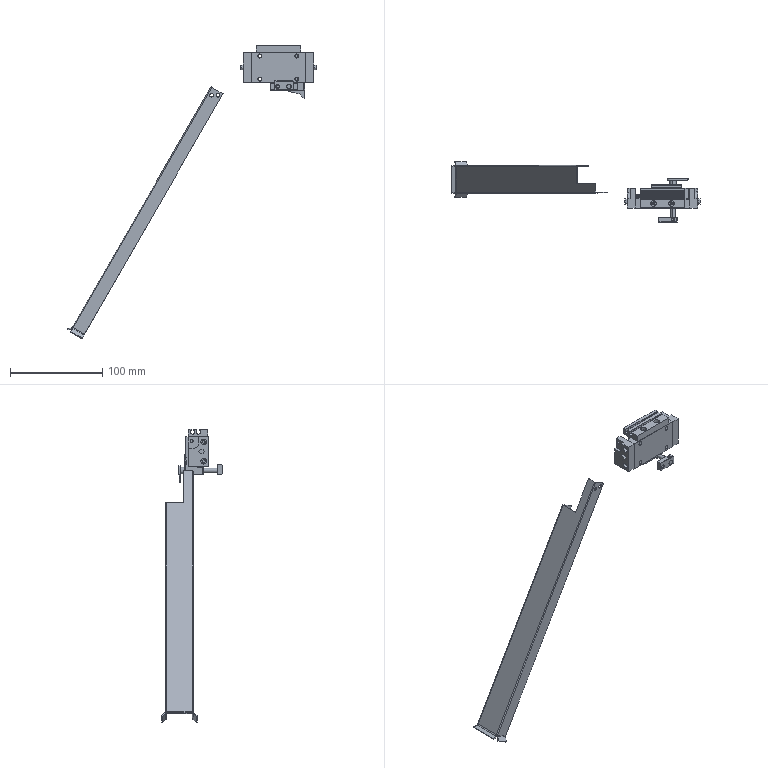Part | NX | 12 solids | 405 faces | box 269.073 x 65.539 x 317.186 mm | volume 76983 mm3 | plane 222 | cylinder 142 | cone 39 | torus 2 | commonest cylinder face diameters 2.5 x20 3.3 x14 6 x14 3.2 x12 4 x8 4.4 x8